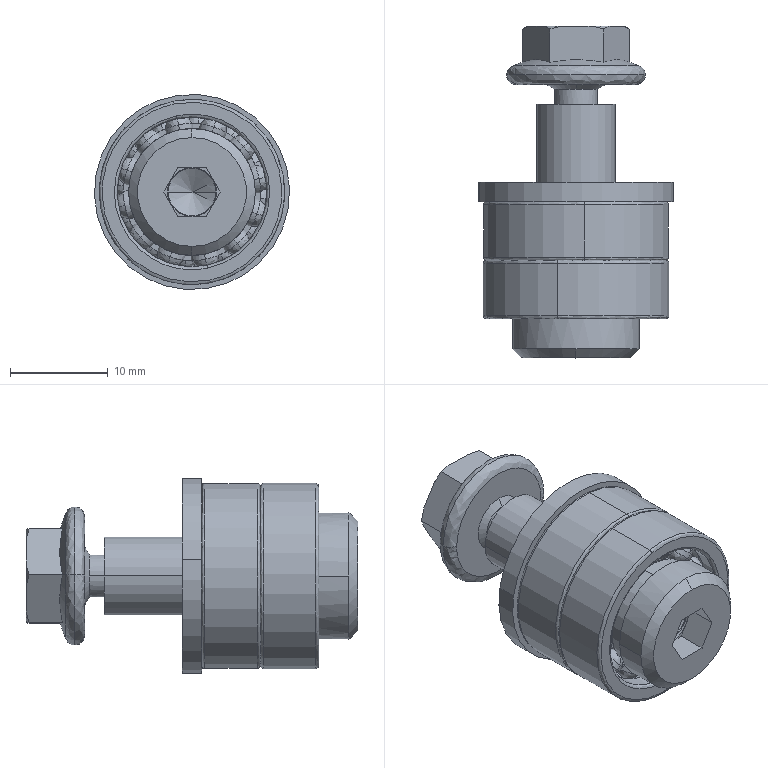Part | SolidWorks | 31 solids | 390 faces | box 20 x 34 x 20 mm | volume 4809 mm3 | spline 152 | cylinder 134 | plane 82 | cone 22 | commonest cylinder face diameters 12.95 x46 14.05 x46 8 x8 11.667 x8 15.333 x8 19 x4